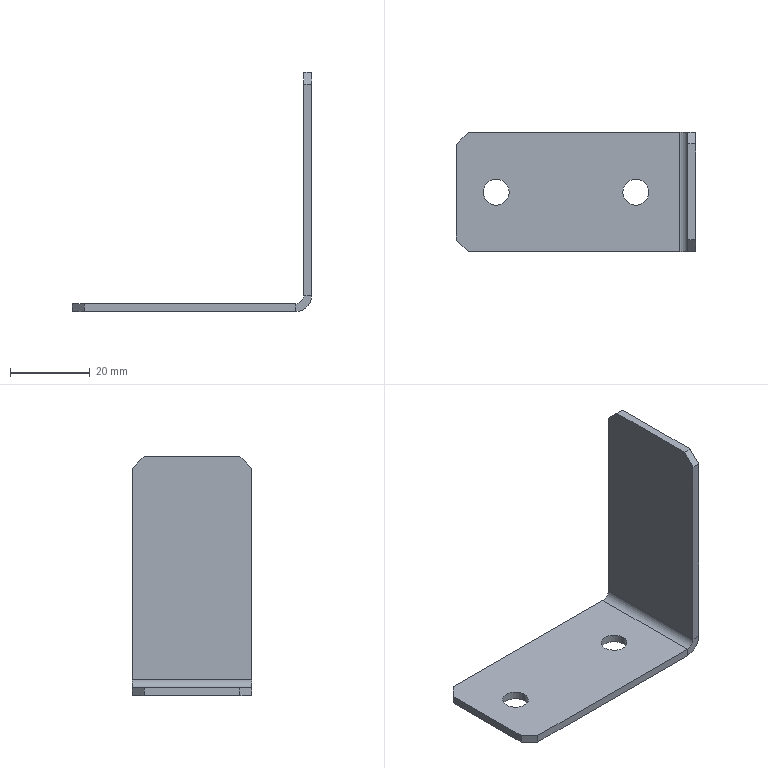Part | SolidWorks | features Chamfer 1, EdgeFlange 1, FlatPattern 1, ICE 1, SMBaseFlange 1, SheetMetal 1 | 1 solid | 22 faces | box 60 x 30 x 60 mm | volume 6834 mm3 | plane 16 | cylinder 6 | commonest cylinder face diameters 6.5 x4 4 x1 8 x1
STEP:
#1=CARTESIAN_POINT('',(-23.25,0.,-2.));
#2=VERTEX_POINT('',#1);
#3=CARTESIAN_POINT('',(-16.75,0.,-2.));
#4=VERTEX_POINT('',#3);
#5=CARTESIAN_POINT('',(-20.,0.,-2.));
#6=DIRECTION('',(0.,0.,1.));
#7=DIRECTION('',(1.,0.,0.));
#8=AXIS2_PLACEMENT_3D('',#5,#6,#7);
#9=CIRCLE('',#8,3.25);
#10=EDGE_CURVE('',#2,#4,#9,.T.);
#11=ORIENTED_EDGE('',*,*,#10,.F.);
#12=CARTESIAN_POINT('',(-23.25,0.,0.));
#13=VERTEX_POINT('',#12);
#14=CARTESIAN_POINT('',(-23.25,0.,-2.));
#15=DIRECTION('',(0.,0.,1.));
#16=VECTOR('',#15,1000.);
#17=LINE('',#14,#16);
#18=EDGE_CURVE('',#2,#13,#17,.T.);
#19=ORIENTED_EDGE('',*,*,#18,.T.);
#20=CARTESIAN_POINT('',(-16.75,0.,0.));
#21=VERTEX_POINT('',#20);
#22=CARTESIAN_POINT('',(-20.,0.,0.));
#23=DIRECTION('',(0.,0.,1.));
#24=DIRECTION('',(1.,0.,0.));
#25=AXIS2_PLACEMENT_3D('',#22,#23,#24);
#26=CIRCLE('',#25,3.25);
#27=EDGE_CURVE('',#13,#21,#26,.T.);
#28=ORIENTED_EDGE('',*,*,#27,.T.);
#29=CARTESIAN_POINT('',(-16.75,0.,-2.));
#30=DIRECTION('',(0.,0.,1.));
#31=VECTOR('',#30,1000.);
#32=LINE('',#29,#31);
#33=EDGE_CURVE('',#4,#21,#32,.T.);
#34=ORIENTED_EDGE('',*,*,#33,.F.);
#35=EDGE_LOOP('',(#11,#19,#28,#34));
#36=FACE_OUTER_BOUND('',#35,.T.);
#37=CARTESIAN_POINT('',(-20.,0.,-2.));
#38=DIRECTION('',(0.,0.,1.));
#39=DIRECTION('',(1.,0.,0.));
#40=AXIS2_PLACEMENT_3D('',#37,#38,#39);
#41=CYLINDRICAL_SURFACE('',#40,3.25);
#42=ADVANCED_FACE('',(#36),#41,.F.);
#43=CARTESIAN_POINT('',(11.75,0.,-2.));
#44=VERTEX_POINT('',#43);
#45=CARTESIAN_POINT('',(18.25,0.,-2.));
#46=VERTEX_POINT('',#45);
#47=CARTESIAN_POINT('',(15.,0.,-2.));
#48=DIRECTION('',(0.,0.,1.));
#49=DIRECTION('',(1.,0.,0.));
#50=AXIS2_PLACEMENT_3D('',#47,#48,#49);
#51=CIRCLE('',#50,3.25);
#52=EDGE_CURVE('',#44,#46,#51,.T.);
#53=ORIENTED_EDGE('',*,*,#52,.F.);
#54=CARTESIAN_POINT('',(11.75,0.,0.));
#55=VERTEX_POINT('',#54);
#56=CARTESIAN_POINT('',(11.75,0.,-2.));
#57=DIRECTION('',(0.,0.,1.));
#58=VECTOR('',#57,1000.);
#59=LINE('',#56,#58);
#60=EDGE_CURVE('',#44,#55,#59,.T.);
#61=ORIENTED_EDGE('',*,*,#60,.T.);
#62=CARTESIAN_POINT('',(18.25,0.,0.));
#63=VERTEX_POINT('',#62);
#64=CARTESIAN_POINT('',(15.,0.,0.));
#65=DIRECTION('',(0.,0.,1.));
#66=DIRECTION('',(1.,0.,0.));
#67=AXIS2_PLACEMENT_3D('',#64,#65,#66);
#68=CIRCLE('',#67,3.25);
#69=EDGE_CURVE('',#55,#63,#68,.T.);
#70=ORIENTED_EDGE('',*,*,#69,.T.);
#71=CARTESIAN_POINT('',(18.25,0.,-2.));
#72=DIRECTION('',(0.,0.,1.));
#73=VECTOR('',#72,1000.);
#74=LINE('',#71,#73);
#75=EDGE_CURVE('',#46,#63,#74,.T.);
#76=ORIENTED_EDGE('',*,*,#75,.F.);
#77=EDGE_LOOP('',(#53,#61,#70,#76));
#78=FACE_OUTER_BOUND('',#77,.T.);
#79=CARTESIAN_POINT('',(15.,0.,-2.));
#80=DIRECTION('',(0.,0.,1.));
#81=DIRECTION('',(1.,0.,0.));
#82=AXIS2_PLACEMENT_3D('',#79,#80,#81);
#83=CYLINDRICAL_SURFACE('',#82,3.25);
#84=ADVANCED_FACE('',(#78),#83,.F.);
#85=CARTESIAN_POINT('',(26.,15.,-2.));
#86=VERTEX_POINT('',#85);
#87=CARTESIAN_POINT('',(-27.,15.,-2.));
#88=VERTEX_POINT('',#87);
#89=CARTESIAN_POINT('',(30.,15.,-2.));
#90=DIRECTION('',(-1.,0.,0.));
#91=VECTOR('',#90,1000.);
#92=LINE('',#89,#91);
#93=EDGE_CURVE('',#86,#88,#92,.T.);
#94=ORIENTED_EDGE('',*,*,#93,.T.);
#95=CARTESIAN_POINT('',(-27.,15.,0.));
#96=VERTEX_POINT('',#95);
#97=CARTESIAN_POINT('',(-27.,15.,-2.));
#98=DIRECTION('',(0.,0.,1.));
#99=VECTOR('',#98,1000.);
#100=LINE('',#97,#99);
#101=EDGE_CURVE('',#88,#96,#100,.T.);
#102=ORIENTED_EDGE('',*,*,#101,.T.);
#103=CARTESIAN_POINT('',(26.,15.,0.));
#104=VERTEX_POINT('',#103);
#105=CARTESIAN_POINT('',(30.,15.,0.));
#106=DIRECTION('',(-1.,0.,0.));
#107=VECTOR('',#106,1000.);
#108=LINE('',#105,#107);
#109=EDGE_CURVE('',#104,#96,#108,.T.);
#110=ORIENTED_EDGE('',*,*,#109,.F.);
#111=CARTESIAN_POINT('',(26.,15.,0.));
#112=DIRECTION('',(0.,0.,-1.));
#113=VECTOR('',#112,1000.);
#114=LINE('',#111,#113);
#115=EDGE_CURVE('',#104,#86,#114,.T.);
#116=ORIENTED_EDGE('',*,*,#115,.T.);
#117=EDGE_LOOP('',(#94,#102,#110,#116));
#118=FACE_OUTER_BOUND('',#117,.T.);
#119=CARTESIAN_POINT('',(30.,15.,-2.));
#120=DIRECTION('',(0.,1.,0.));
#121=DIRECTION('',(-1.,0.,0.));
#122=AXIS2_PLACEMENT_3D('',#119,#120,#121);
#123=PLANE('',#122);
#124=ADVANCED_FACE('',(#118),#123,.T.);
#125=CARTESIAN_POINT('',(-20.,0.,-2.));
#126=DIRECTION('',(0.,0.,1.));
#127=DIRECTION('',(1.,0.,0.));
#128=AXIS2_PLACEMENT_3D('',#125,#126,#127);
#129=CIRCLE('',#128,3.25);
#130=EDGE_CURVE('',#4,#2,#129,.T.);
#131=ORIENTED_EDGE('',*,*,#130,.T.);
#132=ORIENTED_EDGE('',*,*,#10,.T.);
#133=EDGE_LOOP('',(#131,#132));
#134=FACE_BOUND('',#133,.T.);
#135=CARTESIAN_POINT('',(15.,0.,-2.));
#136=DIRECTION('',(0.,0.,1.));
#137=DIRECTION('',(1.,0.,0.));
#138=AXIS2_PLACEMENT_3D('',#135,#136,#137);
#139=CIRCLE('',#138,3.25);
#140=EDGE_CURVE('',#46,#44,#139,.T.);
#141=ORIENTED_EDGE('',*,*,#140,.T.);
#142=ORIENTED_EDGE('',*,*,#52,.T.);
#143=EDGE_LOOP('',(#141,#142));
#144=FACE_BOUND('',#143,.T.);
#145=CARTESIAN_POINT('',(-27.,-15.,-2.));
#146=VERTEX_POINT('',#145);
#147=CARTESIAN_POINT('',(26.,-15.,-2.));
#148=VERTEX_POINT('',#147);
#149=CARTESIAN_POINT('',(30.,-15.,-2.));
#150=DIRECTION('',(1.,0.,0.));
#151=VECTOR('',#150,1000.);
#152=LINE('',#149,#151);
#153=EDGE_CURVE('',#146,#148,#152,.T.);
#154=ORIENTED_EDGE('',*,*,#153,.F.);
#155=CARTESIAN_POINT('',(-30.,-12.,-2.));
#156=VERTEX_POINT('',#155);
#157=CARTESIAN_POINT('',(-30.,-12.,-2.));
#158=DIRECTION('',(-0.7071,0.7071,0.));
#159=VECTOR('',#158,1000.);
#160=LINE('',#157,#159);
#161=EDGE_CURVE('',#146,#156,#160,.T.);
#162=ORIENTED_EDGE('',*,*,#161,.T.);
#163=CARTESIAN_POINT('',(-30.,12.,-2.));
#164=VERTEX_POINT('',#163);
#165=CARTESIAN_POINT('',(-30.,-15.,-2.));
#166=DIRECTION('',(0.,-1.,0.));
#167=VECTOR('',#166,1000.);
#168=LINE('',#165,#167);
#169=EDGE_CURVE('',#164,#156,#168,.T.);
#170=ORIENTED_EDGE('',*,*,#169,.F.);
#171=CARTESIAN_POINT('',(-27.,15.,-2.));
#172=DIRECTION('',(0.7071,0.7071,0.));
#173=VECTOR('',#172,1000.);
#174=LINE('',#171,#173);
#175=EDGE_CURVE('',#164,#88,#174,.T.);
#176=ORIENTED_EDGE('',*,*,#175,.T.);
#177=ORIENTED_EDGE('',*,*,#93,.F.);
#178=CARTESIAN_POINT('',(26.,15.,-2.));
#179=DIRECTION('',(0.,-1.,0.));
#180=VECTOR('',#179,1000.);
#181=LINE('',#178,#180);
#182=EDGE_CURVE('',#86,#148,#181,.T.);
#183=ORIENTED_EDGE('',*,*,#182,.T.);
#184=EDGE_LOOP('',(#154,#162,#170,#176,#177,#183));
#185=FACE_OUTER_BOUND('',#184,.T.);
#186=CARTESIAN_POINT('',(0.,0.,-2.));
#187=DIRECTION('',(0.,0.,1.));
#188=DIRECTION('',(1.,0.,0.));
#189=AXIS2_PLACEMENT_3D('',#186,#187,#188);
#190=PLANE('',#189);
#191=ADVANCED_FACE('',(#134,#144,#185),#190,.F.);
#192=CARTESIAN_POINT('',(-20.,0.,0.));
#193=DIRECTION('',(0.,0.,1.));
#194=DIRECTION('',(1.,0.,0.));
#195=AXIS2_PLACEMENT_3D('',#192,#193,#194);
#196=CIRCLE('',#195,3.25);
#197=EDGE_CURVE('',#21,#13,#196,.T.);
#198=ORIENTED_EDGE('',*,*,#197,.F.);
#199=ORIENTED_EDGE('',*,*,#27,.F.);
#200=EDGE_LOOP('',(#198,#199));
#201=FACE_BOUND('',#200,.T.);
#202=CARTESIAN_POINT('',(15.,0.,0.));
#203=DIRECTION('',(0.,0.,1.));
#204=DIRECTION('',(1.,0.,0.));
#205=AXIS2_PLACEMENT_3D('',#202,#203,#204);
#206=CIRCLE('',#205,3.25);
#207=EDGE_CURVE('',#63,#55,#206,.T.);
#208=ORIENTED_EDGE('',*,*,#207,.F.);
#209=ORIENTED_EDGE('',*,*,#69,.F.);
#210=EDGE_LOOP('',(#208,#209));
#211=FACE_BOUND('',#210,.T.);
#212=CARTESIAN_POINT('',(-30.,12.,0.));
#213=VERTEX_POINT('',#212);
#214=CARTESIAN_POINT('',(-30.,-12.,0.));
#215=VERTEX_POINT('',#214);
#216=CARTESIAN_POINT('',(-30.,-15.,0.));
#217=DIRECTION('',(0.,-1.,0.));
#218=VECTOR('',#217,1000.);
#219=LINE('',#216,#218);
#220=EDGE_CURVE('',#213,#215,#219,.T.);
#221=ORIENTED_EDGE('',*,*,#220,.T.);
#222=CARTESIAN_POINT('',(-27.,-15.,0.));
#223=VERTEX_POINT('',#222);
#224=CARTESIAN_POINT('',(-21.,-21.,0.));
#225=DIRECTION('',(0.7071,-0.7071,0.));
#226=VECTOR('',#225,1000.);
#227=LINE('',#224,#226);
#228=EDGE_CURVE('',#215,#223,#227,.T.);
#229=ORIENTED_EDGE('',*,*,#228,.T.);
#230=CARTESIAN_POINT('',(26.,-15.,0.));
#231=VERTEX_POINT('',#230);
#232=CARTESIAN_POINT('',(30.,-15.,0.));
#233=DIRECTION('',(1.,0.,0.));
#234=VECTOR('',#233,1000.);
#235=LINE('',#232,#234);
#236=EDGE_CURVE('',#223,#231,#235,.T.);
#237=ORIENTED_EDGE('',*,*,#236,.T.);
#238=CARTESIAN_POINT('',(26.,15.,0.));
#239=DIRECTION('',(0.,-1.,0.));
#240=VECTOR('',#239,1000.);
#241=LINE('',#238,#240);
#242=EDGE_CURVE('',#104,#231,#241,.T.);
#243=ORIENTED_EDGE('',*,*,#242,.F.);
#244=ORIENTED_EDGE('',*,*,#109,.T.);
#245=CARTESIAN_POINT('',(-21.,21.,0.));
#246=DIRECTION('',(-0.7071,-0.7071,0.));
#247=VECTOR('',#246,1000.);
#248=LINE('',#245,#247);
#249=EDGE_CURVE('',#96,#213,#248,.T.);
#250=ORIENTED_EDGE('',*,*,#249,.T.);
#251=EDGE_LOOP('',(#221,#229,#237,#243,#244,#250));
#252=FACE_OUTER_BOUND('',#251,.T.);
#253=CARTESIAN_POINT('',(0.,0.,0.));
#254=DIRECTION('',(0.,0.,1.));
#255=DIRECTION('',(1.,0.,0.));
#256=AXIS2_PLACEMENT_3D('',#253,#254,#255);
#257=PLANE('',#256);
#258=ADVANCED_FACE('',(#201,#211,#252),#257,.T.);
#259=ORIENTED_EDGE('',*,*,#169,.T.);
#260=CARTESIAN_POINT('',(-30.,-12.,-2.));
#261=DIRECTION('',(0.,0.,1.));
#262=VECTOR('',#261,1000.);
#263=LINE('',#260,#262);
#264=EDGE_CURVE('',#156,#215,#263,.T.);
#265=ORIENTED_EDGE('',*,*,#264,.T.);
#266=ORIENTED_EDGE('',*,*,#220,.F.);
#267=CARTESIAN_POINT('',(-30.,12.,-2.));
#268=DIRECTION('',(0.,0.,-1.));
#269=VECTOR('',#268,1000.);
#270=LINE('',#267,#269);
#271=EDGE_CURVE('',#213,#164,#270,.T.);
#272=ORIENTED_EDGE('',*,*,#271,.T.);
#273=EDGE_LOOP('',(#259,#265,#266,#272));
#274=FACE_OUTER_BOUND('',#273,.T.);
#275=CARTESIAN_POINT('',(-30.,-15.,-2.));
#276=DIRECTION('',(-1.,0.,0.));
#277=DIRECTION('',(0.,0.,1.));
#278=AXIS2_PLACEMENT_3D('',#275,#276,#277);
#279=PLANE('',#278);
#280=ADVANCED_FACE('',(#274),#279,.T.);
#281=ORIENTED_EDGE('',*,*,#236,.F.);
#282=CARTESIAN_POINT('',(-27.,-15.,-2.));
#283=DIRECTION('',(0.,0.,-1.));
#284=VECTOR('',#283,1000.);
#285=LINE('',#282,#284);
#286=EDGE_CURVE('',#223,#146,#285,.T.);
#287=ORIENTED_EDGE('',*,*,#286,.T.);
#288=ORIENTED_EDGE('',*,*,#153,.T.);
#289=CARTESIAN_POINT('',(26.,-15.,0.));
#290=DIRECTION('',(0.,0.,-1.));
#291=VECTOR('',#290,1000.);
#292=LINE('',#289,#291);
#293=EDGE_CURVE('',#231,#148,#292,.T.);
#294=ORIENTED_EDGE('',*,*,#293,.F.);
#295=EDGE_LOOP('',(#281,#287,#288,#294));
#296=FACE_OUTER_BOUND('',#295,.T.);
#297=CARTESIAN_POINT('',(30.,-15.,-2.));
#298=DIRECTION('',(0.,-1.,0.));
#299=DIRECTION('',(1.,0.,0.));
#300=AXIS2_PLACEMENT_3D('',#297,#298,#299);
#301=PLANE('',#300);
#302=ADVANCED_FACE('',(#296),#301,.T.);
#303=CARTESIAN_POINT('',(28.,-15.,2.));
#304=VERTEX_POINT('',#303);
#305=CARTESIAN_POINT('',(30.,-15.,2.));
#306=VERTEX_POINT('',#305);
#307=CARTESIAN_POINT('',(30.,-15.,2.));
#308=DIRECTION('',(1.,0.,0.));
#309=VECTOR('',#308,1000.);
#310=LINE('',#307,#309);
#311=EDGE_CURVE('',#304,#306,#310,.T.);
#312=ORIENTED_EDGE('',*,*,#311,.F.);
#313=CARTESIAN_POINT('',(26.,-15.,2.));
#314=DIRECTION('',(0.,-1.,0.));
#315=DIRECTION('',(0.,0.,1.));
#316=AXIS2_PLACEMENT_3D('',#313,#314,#315);
#317=CIRCLE('',#316,2.);
#318=EDGE_CURVE('',#231,#304,#317,.T.);
#319=ORIENTED_EDGE('',*,*,#318,.F.);
#320=ORIENTED_EDGE('',*,*,#293,.T.);
#321=CARTESIAN_POINT('',(26.,-15.,2.));
#322=DIRECTION('',(0.,-1.,0.));
#323=DIRECTION('',(0.,0.,1.));
#324=AXIS2_PLACEMENT_3D('',#321,#322,#323);
#325=CIRCLE('',#324,4.);
#326=EDGE_CURVE('',#148,#306,#325,.T.);
#327=ORIENTED_EDGE('',*,*,#326,.T.);
#328=EDGE_LOOP('',(#312,#319,#320,#327));
#329=FACE_OUTER_BOUND('',#328,.T.);
#330=CARTESIAN_POINT('',(26.,-15.,2.));
#331=DIRECTION('',(0.,-1.,0.));
#332=DIRECTION('',(0.,0.,-1.));
#333=AXIS2_PLACEMENT_3D('',#330,#331,#332);
#334=PLANE('',#333);
#335=ADVANCED_FACE('',(#329),#334,.T.);
#336=CARTESIAN_POINT('',(28.,15.,2.));
#337=VERTEX_POINT('',#336);
#338=CARTESIAN_POINT('',(26.,15.,2.));
#339=DIRECTION('',(0.,1.,0.));
#340=DIRECTION('',(0.,0.,1.));
#341=AXIS2_PLACEMENT_3D('',#338,#339,#340);
#342=CIRCLE('',#341,2.);
#343=EDGE_CURVE('',#337,#104,#342,.T.);
#344=ORIENTED_EDGE('',*,*,#343,.F.);
#345=CARTESIAN_POINT('',(30.,15.,2.));
#346=VERTEX_POINT('',#345);
#347=CARTESIAN_POINT('',(28.,15.,2.));
#348=DIRECTION('',(1.,0.,0.));
#349=VECTOR('',#348,1000.);
#350=LINE('',#347,#349);
#351=EDGE_CURVE('',#337,#346,#350,.T.);
#352=ORIENTED_EDGE('',*,*,#351,.T.);
#353=CARTESIAN_POINT('',(26.,15.,2.));
#354=DIRECTION('',(0.,1.,0.));
#355=DIRECTION('',(0.,0.,1.));
#356=AXIS2_PLACEMENT_3D('',#353,#354,#355);
#357=CIRCLE('',#356,4.);
#358=EDGE_CURVE('',#346,#86,#357,.T.);
#359=ORIENTED_EDGE('',*,*,#358,.T.);
#360=ORIENTED_EDGE('',*,*,#115,.F.);
#361=EDGE_LOOP('',(#344,#352,#359,#360));
#362=FACE_OUTER_BOUND('',#361,.T.);
#363=CARTESIAN_POINT('',(26.,15.,2.));
#364=DIRECTION('',(0.,-1.,0.));
#365=DIRECTION('',(0.,0.,-1.));
#366=AXIS2_PLACEMENT_3D('',#363,#364,#365);
#367=PLANE('',#366);
#368=ADVANCED_FACE('',(#362),#367,.F.);
#369=ORIENTED_EDGE('',*,*,#182,.F.);
#370=ORIENTED_EDGE('',*,*,#358,.F.);
#371=CARTESIAN_POINT('',(30.,0.,2.));
#372=DIRECTION('',(0.,1.,0.));
#373=VECTOR('',#372,1000.);
#374=LINE('',#371,#373);
#375=EDGE_CURVE('',#306,#346,#374,.T.);
#376=ORIENTED_EDGE('',*,*,#375,.F.);
#377=ORIENTED_EDGE('',*,*,#326,.F.);
#378=EDGE_LOOP('',(#369,#370,#376,#377));
#379=FACE_OUTER_BOUND('',#378,.T.);
#380=CARTESIAN_POINT('',(26.,15.,2.));
#381=DIRECTION('',(0.,1.,0.));
#382=DIRECTION('',(1.,0.,0.));
#383=AXIS2_PLACEMENT_3D('',#380,#381,#382);
#384=CYLINDRICAL_SURFACE('',#383,4.);
#385=ADVANCED_FACE('',(#379),#384,.T.);
#386=ORIENTED_EDGE('',*,*,#242,.T.);
#387=ORIENTED_EDGE('',*,*,#318,.T.);
#388=CARTESIAN_POINT('',(28.,-15.,2.));
#389=DIRECTION('',(0.,1.,0.));
#390=VECTOR('',#389,1000.);
#391=LINE('',#388,#390);
#392=EDGE_CURVE('',#304,#337,#391,.T.);
#393=ORIENTED_EDGE('',*,*,#392,.T.);
#394=ORIENTED_EDGE('',*,*,#343,.T.);
#395=EDGE_LOOP('',(#386,#387,#393,#394));
#396=FACE_OUTER_BOUND('',#395,.T.);
#397=CARTESIAN_POINT('',(26.,15.,2.));
#398=DIRECTION('',(0.,1.,0.));
#399=DIRECTION('',(1.,0.,0.));
#400=AXIS2_PLACEMENT_3D('',#397,#398,#399);
#401=CYLINDRICAL_SURFACE('',#400,2.);
#402=ADVANCED_FACE('',(#396),#401,.F.);
#403=CARTESIAN_POINT('',(28.,15.,55.));
#404=VERTEX_POINT('',#403);
#405=CARTESIAN_POINT('',(28.,15.,0.));
#406=DIRECTION('',(0.,0.,-1.));
#407=VECTOR('',#406,1000.);
#408=LINE('',#405,#407);
#409=EDGE_CURVE('',#404,#337,#408,.T.);
#410=ORIENTED_EDGE('',*,*,#409,.F.);
#411=CARTESIAN_POINT('',(30.,15.,55.));
#412=VERTEX_POINT('',#411);
#413=CARTESIAN_POINT('',(30.,15.,55.));
#414=DIRECTION('',(1.,0.,0.));
#415=VECTOR('',#414,1000.);
#416=LINE('',#413,#415);
#417=EDGE_CURVE('',#404,#412,#416,.T.);
#418=ORIENTED_EDGE('',*,*,#417,.T.);
#419=CARTESIAN_POINT('',(30.,15.,0.));
#420=DIRECTION('',(0.,0.,-1.));
#421=VECTOR('',#420,1000.);
#422=LINE('',#419,#421);
#423=EDGE_CURVE('',#412,#346,#422,.T.);
#424=ORIENTED_EDGE('',*,*,#423,.T.);
#425=ORIENTED_EDGE('',*,*,#351,.F.);
#426=EDGE_LOOP('',(#410,#418,#424,#425));
#427=FACE_OUTER_BOUND('',#426,.T.);
#428=CARTESIAN_POINT('',(30.,15.,0.));
#429=DIRECTION('',(0.,1.,0.));
#430=DIRECTION('',(0.,0.,1.));
#431=AXIS2_PLACEMENT_3D('',#428,#429,#430);
#432=PLANE('',#431);
#433=ADVANCED_FACE('',(#427),#432,.T.);
#434=CARTESIAN_POINT('',(30.,-15.,55.));
#435=VERTEX_POINT('',#434);
#436=CARTESIAN_POINT('',(30.,-15.,58.));
#437=DIRECTION('',(0.,0.,1.));
#438=VECTOR('',#437,1000.);
#439=LINE('',#436,#438);
#440=EDGE_CURVE('',#306,#435,#439,.T.);
#441=ORIENTED_EDGE('',*,*,#440,.T.);
#442=CARTESIAN_POINT('',(28.,-15.,55.));
#443=VERTEX_POINT('',#442);
#444=CARTESIAN_POINT('',(30.,-15.,55.));
#445=DIRECTION('',(-1.,0.,0.));
#446=VECTOR('',#445,1000.);
#447=LINE('',#444,#446);
#448=EDGE_CURVE('',#435,#443,#447,.T.);
#449=ORIENTED_EDGE('',*,*,#448,.T.);
#450=CARTESIAN_POINT('',(28.,-15.,0.));
#451=DIRECTION('',(0.,0.,1.));
#452=VECTOR('',#451,1000.);
#453=LINE('',#450,#452);
#454=EDGE_CURVE('',#304,#443,#453,.T.);
#455=ORIENTED_EDGE('',*,*,#454,.F.);
#456=ORIENTED_EDGE('',*,*,#311,.T.);
#457=EDGE_LOOP('',(#441,#449,#455,#456));
#458=FACE_OUTER_BOUND('',#457,.T.);
#459=CARTESIAN_POINT('',(30.,-15.,58.));
#460=DIRECTION('',(0.,-1.,0.));
#461=DIRECTION('',(0.,0.,-1.));
#462=AXIS2_PLACEMENT_3D('',#459,#460,#461);
#463=PLANE('',#462);
#464=ADVANCED_FACE('',(#458),#463,.T.);
#465=ORIENTED_EDGE('',*,*,#423,.F.);
#466=CARTESIAN_POINT('',(30.,12.,58.));
#467=VERTEX_POINT('',#466);
#468=CARTESIAN_POINT('',(30.,35.,35.));
#469=DIRECTION('',(0.,-0.7071,0.7071));
#470=VECTOR('',#469,1000.);
#471=LINE('',#468,#470);
#472=EDGE_CURVE('',#412,#467,#471,.T.);
#473=ORIENTED_EDGE('',*,*,#472,.T.);
#474=CARTESIAN_POINT('',(30.,-12.,58.));
#475=VERTEX_POINT('',#474);
#476=CARTESIAN_POINT('',(30.,15.,58.));
#477=DIRECTION('',(0.,1.,0.));
#478=VECTOR('',#477,1000.);
#479=LINE('',#476,#478);
#480=EDGE_CURVE('',#475,#467,#479,.T.);
#481=ORIENTED_EDGE('',*,*,#480,.F.);
#482=CARTESIAN_POINT('',(30.,-35.,35.));
#483=DIRECTION('',(0.,-0.7071,-0.7071));
#484=VECTOR('',#483,1000.);
#485=LINE('',#482,#484);
#486=EDGE_CURVE('',#475,#435,#485,.T.);
#487=ORIENTED_EDGE('',*,*,#486,.T.);
#488=ORIENTED_EDGE('',*,*,#440,.F.);
#489=ORIENTED_EDGE('',*,*,#375,.T.);
#490=EDGE_LOOP('',(#465,#473,#481,#487,#488,#489));
#491=FACE_OUTER_BOUND('',#490,.T.);
#492=CARTESIAN_POINT('',(30.,0.,0.));
#493=DIRECTION('',(1.,0.,0.));
#494=DIRECTION('',(0.,0.,-1.));
#495=AXIS2_PLACEMENT_3D('',#492,#493,#494);
#496=PLANE('',#495);
#497=ADVANCED_FACE('',(#491),#496,.T.);
#498=CARTESIAN_POINT('',(28.,-12.,58.));
#499=VERTEX_POINT('',#498);
#500=CARTESIAN_POINT('',(28.,12.,58.));
#501=VERTEX_POINT('',#500);
#502=CARTESIAN_POINT('',(28.,0.,58.));
#503=DIRECTION('',(0.,1.,0.));
#504=VECTOR('',#503,1000.);
#505=LINE('',#502,#504);
#506=EDGE_CURVE('',#499,#501,#505,.T.);
#507=ORIENTED_EDGE('',*,*,#506,.T.);
#508=CARTESIAN_POINT('',(28.,12.,58.));
#509=DIRECTION('',(0.,0.7071,-0.7071));
#510=VECTOR('',#509,1000.);
#511=LINE('',#508,#510);
#512=EDGE_CURVE('',#501,#404,#511,.T.);
#513=ORIENTED_EDGE('',*,*,#512,.T.);
#514=ORIENTED_EDGE('',*,*,#409,.T.);
#515=ORIENTED_EDGE('',*,*,#392,.F.);
#516=ORIENTED_EDGE('',*,*,#454,.T.);
#517=CARTESIAN_POINT('',(28.,-15.,55.));
#518=DIRECTION('',(0.,0.7071,0.7071));
#519=VECTOR('',#518,1000.);
#520=LINE('',#517,#519);
#521=EDGE_CURVE('',#443,#499,#520,.T.);
#522=ORIENTED_EDGE('',*,*,#521,.T.);
#523=EDGE_LOOP('',(#507,#513,#514,#515,#516,#522));
#524=FACE_OUTER_BOUND('',#523,.T.);
#525=CARTESIAN_POINT('',(28.,0.,0.));
#526=DIRECTION('',(1.,0.,0.));
#527=DIRECTION('',(0.,0.,-1.));
#528=AXIS2_PLACEMENT_3D('',#525,#526,#527);
#529=PLANE('',#528);
#530=ADVANCED_FACE('',(#524),#529,.F.);
#531=ORIENTED_EDGE('',*,*,#480,.T.);
#532=CARTESIAN_POINT('',(30.,12.,58.));
#533=DIRECTION('',(-1.,0.,0.));
#534=VECTOR('',#533,1000.);
#535=LINE('',#532,#534);
#536=EDGE_CURVE('',#467,#501,#535,.T.);
#537=ORIENTED_EDGE('',*,*,#536,.T.);
#538=ORIENTED_EDGE('',*,*,#506,.F.);
#539=CARTESIAN_POINT('',(30.,-12.,58.));
#540=DIRECTION('',(1.,0.,0.));
#541=VECTOR('',#540,1000.);
#542=LINE('',#539,#541);
#543=EDGE_CURVE('',#499,#475,#542,.T.);
#544=ORIENTED_EDGE('',*,*,#543,.T.);
#545=EDGE_LOOP('',(#531,#537,#538,#544));
#546=FACE_OUTER_BOUND('',#545,.T.);
#547=CARTESIAN_POINT('',(30.,15.,58.));
#548=DIRECTION('',(0.,0.,1.));
#549=DIRECTION('',(1.,0.,0.));
#550=AXIS2_PLACEMENT_3D('',#547,#548,#549);
#551=PLANE('',#550);
#552=ADVANCED_FACE('',(#546),#551,.T.);
#553=ORIENTED_EDGE('',*,*,#472,.F.);
#554=ORIENTED_EDGE('',*,*,#417,.F.);
#555=ORIENTED_EDGE('',*,*,#512,.F.);
#556=ORIENTED_EDGE('',*,*,#536,.F.);
#557=EDGE_LOOP('',(#553,#554,#555,#556));
#558=FACE_OUTER_BOUND('',#557,.T.);
#559=CARTESIAN_POINT('',(30.,12.,58.));
#560=DIRECTION('',(0.,-0.7071,-0.7071));
#561=DIRECTION('',(-1.,0.,0.));
#562=AXIS2_PLACEMENT_3D('',#559,#560,#561);
#563=PLANE('',#562);
#564=ADVANCED_FACE('',(#558),#563,.F.);
#565=ORIENTED_EDGE('',*,*,#486,.F.);
#566=ORIENTED_EDGE('',*,*,#543,.F.);
#567=ORIENTED_EDGE('',*,*,#521,.F.);
#568=ORIENTED_EDGE('',*,*,#448,.F.);
#569=EDGE_LOOP('',(#565,#566,#567,#568));
#570=FACE_OUTER_BOUND('',#569,.T.);
#571=CARTESIAN_POINT('',(30.,-15.,55.));
#572=DIRECTION('',(0.,0.7071,-0.7071));
#573=DIRECTION('',(-1.,0.,0.));
#574=AXIS2_PLACEMENT_3D('',#571,#572,#573);
#575=PLANE('',#574);
#576=ADVANCED_FACE('',(#570),#575,.F.);
#577=ORIENTED_EDGE('',*,*,#161,.F.);
#578=ORIENTED_EDGE('',*,*,#286,.F.);
#579=ORIENTED_EDGE('',*,*,#228,.F.);
#580=ORIENTED_EDGE('',*,*,#264,.F.);
#581=EDGE_LOOP('',(#577,#578,#579,#580));
#582=FACE_OUTER_BOUND('',#581,.T.);
#583=CARTESIAN_POINT('',(-30.,-12.,-2.));
#584=DIRECTION('',(0.7071,0.7071,0.));
#585=DIRECTION('',(0.,0.,1.));
#586=AXIS2_PLACEMENT_3D('',#583,#584,#585);
#587=PLANE('',#586);
#588=ADVANCED_FACE('',(#582),#587,.F.);
#589=ORIENTED_EDGE('',*,*,#175,.F.);
#590=ORIENTED_EDGE('',*,*,#271,.F.);
#591=ORIENTED_EDGE('',*,*,#249,.F.);
#592=ORIENTED_EDGE('',*,*,#101,.F.);
#593=EDGE_LOOP('',(#589,#590,#591,#592));
#594=FACE_OUTER_BOUND('',#593,.T.);
#595=CARTESIAN_POINT('',(-27.,15.,-2.));
#596=DIRECTION('',(0.7071,-0.7071,0.));
#597=DIRECTION('',(0.,0.,1.));
#598=AXIS2_PLACEMENT_3D('',#595,#596,#597);
#599=PLANE('',#598);
#600=ADVANCED_FACE('',(#594),#599,.F.);
#601=ORIENTED_EDGE('',*,*,#60,.F.);
#602=ORIENTED_EDGE('',*,*,#140,.F.);
#603=ORIENTED_EDGE('',*,*,#75,.T.);
#604=ORIENTED_EDGE('',*,*,#207,.T.);
#605=EDGE_LOOP('',(#601,#602,#603,#604));
#606=FACE_OUTER_BOUND('',#605,.T.);
#607=CARTESIAN_POINT('',(15.,0.,-2.));
#608=DIRECTION('',(0.,0.,1.));
#609=DIRECTION('',(1.,0.,0.));
#610=AXIS2_PLACEMENT_3D('',#607,#608,#609);
#611=CYLINDRICAL_SURFACE('',#610,3.25);
#612=ADVANCED_FACE('',(#606),#611,.F.);
#613=ORIENTED_EDGE('',*,*,#18,.F.);
#614=ORIENTED_EDGE('',*,*,#130,.F.);
#615=ORIENTED_EDGE('',*,*,#33,.T.);
#616=ORIENTED_EDGE('',*,*,#197,.T.);
#617=EDGE_LOOP('',(#613,#614,#615,#616));
#618=FACE_OUTER_BOUND('',#617,.T.);
#619=CARTESIAN_POINT('',(-20.,0.,-2.));
#620=DIRECTION('',(0.,0.,1.));
#621=DIRECTION('',(1.,0.,0.));
#622=AXIS2_PLACEMENT_3D('',#619,#620,#621);
#623=CYLINDRICAL_SURFACE('',#622,3.25);
#624=ADVANCED_FACE('',(#618),#623,.F.);
#625=CLOSED_SHELL('',(#42,#84,#124,#191,#258,#280,#302,#335,#368,#385,#402,#433,#464,#497,#530,#552,#564,#576,#588,#600,#612,#624));
#626=MANIFOLD_SOLID_BREP('',#625);
#627=CARTESIAN_POINT('',(0.,0.,0.));
#628=DIRECTION('',(0.,0.,1.));
#629=DIRECTION('',(1.,0.,0.));
#630=AXIS2_PLACEMENT_3D('',#627,#628,#629);
#631=(LENGTH_UNIT()NAMED_UNIT(*)SI_UNIT(.MILLI.,.METRE.));
#632=UNCERTAINTY_MEASURE_WITH_UNIT(LENGTH_MEASURE(0.00001),#631,'','');
#633=(NAMED_UNIT(*)PLANE_ANGLE_UNIT()SI_UNIT($,.RADIAN.));
#634=(NAMED_UNIT(*)SI_UNIT($,.STERADIAN.)SOLID_ANGLE_UNIT());
#635=(GEOMETRIC_REPRESENTATION_CONTEXT(3)GLOBAL_UNCERTAINTY_ASSIGNED_CONTEXT((#632))GLOBAL_UNIT_ASSIGNED_CONTEXT((#631,#633,#634))REPRESENTATION_CONTEXT('',''));
#636=ADVANCED_BREP_SHAPE_REPRESENTATION('',(#626,#630),#635);